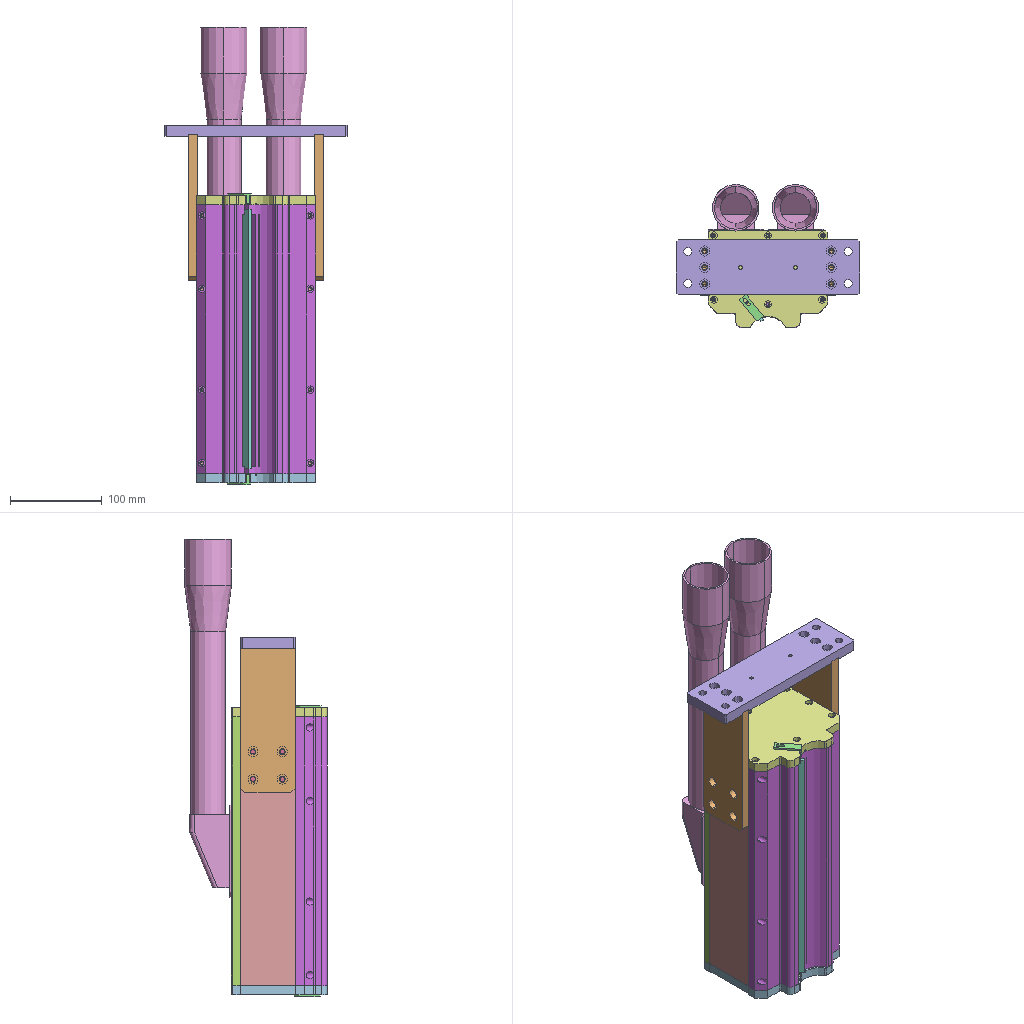Assembly | SolidWorks | 12 different items | 16 placed | box 200 x 156 x 499 mm
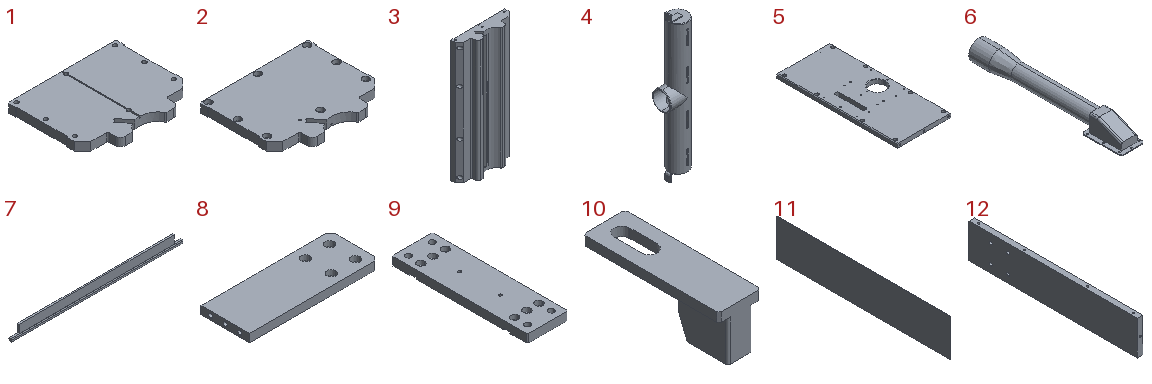Parts list (item | quantity | size | volume | features):
1 | x1 | 130 x 105 x 10 mm | 118021 mm3 | features ICE 5, Fillet 3, Chamfer 2, HoleWzd 2, Extrusion 1
2 | x1 | 130 x 105 x 10 mm | 118021 mm3 | features ICE 5, Fillet 3, Chamfer 2, HoleWzd 2, Extrusion 1
3 | x1 | 130 x 35 x 293 mm | 778685 mm3 | features ICE 4, Fillet 3, HoleWzd 2, MirrorPattern 2, Chamfer 1, Cut 1, Extrusion 1, LPattern 1
4 | x1 | 52 x 38 x 290 mm | 64495 mm3 | features Fillet 4, ICE 4, Chamfer 3, MirrorPattern 2, Extrusion 1, Shell 1
5 | x1 | 130 x 293 x 10 mm | 356054 mm3 | features HoleWzd 5, MirrorPattern 4, Chamfer 2, Cut 2, Extrusion 1, ICE 1
6 | x2 | 60 x 390 x 51 mm | 98660 mm3 | features ICE 4, Chamfer 1, Cut 1, Extrusion 1, Fillet 1, MirrorPattern 1, Revolution 1, Shell 1
7 | x1 | 313 x 5 x 20.5 mm | 20756 mm3 | features ICE 2, Extrusion 1
8 | x2 | 160 x 60 x 10 mm | 92147 mm3 | features HoleWzd 2, Chamfer 1, Extrusion 1
9 | x1 | 60 x 200 x 12 mm | 134076 mm3 | features Cut 2, Chamfer 1, Extrusion 1, HoleWzd 1, ICE 1
10 | x2 | 9.3 x 30 x 11 mm | 992.992 mm3 | features Chamfer 2, ICE 2, Extrusion 1, Fillet 1
11 | x1 | 1.5 x 297 x 64 mm | 28512 mm3 | features Extrusion 1
12 | x2 | 10 x 293 x 60 mm | 174003 mm3 | features HoleWzd 3, MirrorPattern 2, Extrusion 1
Mates (type | each side: item.copy, entity, surface, feature):
Coincident | 3.1 plane | 11.1 plane
Coincident | 3.1 face plane Boss-Extrude1 | 12.1 face plane Boss-Extrude1
Coincident | 3.1 face plane Boss-Extrude1 | 12.2 face plane Boss-Extrude1
Coincident | 3.1 face plane Boss-Extrude1 | 2.1 face plane Boss-Extrude1
Coincident | 3.1 plane | 4.1 plane
Coincident | 3.1 face plane Boss-Extrude1 | 1.1 face plane Boss-Extrude1
Coincident | 12.1 face plane Boss-Extrude1 | 5.1 face plane Boss-Extrude1 | 2 times
Coincident | 5.1 face plane Boss-Extrude1 | 6.1 face plane Boss-Extrude1
Coincident | 1.1 face plane Cut-Extrude8 | 7.1 face plane Boss-Extrude1 | 2 times
Coincident | 1.1 face plane Boss-Extrude1 | 7.1 face plane Boss-Extrude1
Coincident | 1.1 plane | 9.1 plane
Coincident | 2.1 face plane Boss-Extrude1 | 5.1 face plane Boss-Extrude1
Coincident | 2.1 face plane Cut-Extrude8 | 10.1 face plane Boss-Extrude1
Coincident | 2.1 face plane Boss-Extrude1 | 10.1 face plane Boss-Extrude2
Coincident | 5.1 plane | 6.1 plane
Coincident | 5.1 face plane Boss-Extrude1 | 6.1 face plane Boss-Extrude3
Coincident | 1.1 face plane Boss-Extrude1 | 10.2 face plane Boss-Extrude2
Coincident | 1.1 face plane Cut-Extrude8 | 10.2 face plane Boss-Extrude1
Coincident | 7.1 face plane Boss-Extrude1 | 10.2 face plane Boss-Extrude1
Coincident | 12.1 face plane Boss-Extrude1 | 2.1 face plane Boss-Extrude1
DistanceDim | 12.1 face plane Boss-Extrude1 | 3.1 face plane Boss-Extrude1
Coincident | 12.2 face plane Boss-Extrude1 | 2.1 face plane Boss-Extrude1
DistanceDim | 12.2 face plane Boss-Extrude1 | 3.1 face plane Boss-Extrude1
Coincident | 5.1 face plane Cut-Extrude3 | 11.1 face plane Boss-Extrude1
DistanceDim | 11.1 face plane Boss-Extrude1 | 5.1 face plane Boss-Extrude1
Coincident | 12.1 face plane Boss-Extrude1 | 8.1 face plane Boss-Extrude1
Concentric | 12.1 face cylinder M6 Tapped Hole1 | 8.1 face cylinder CBORE for M6 Hex Socket Head Cap Screw1 | 2 times
Coincident | 12.2 face plane Boss-Extrude1 | 8.2 face plane Boss-Extrude1
Concentric | 12.2 face cylinder M6 Tapped Hole1 | 8.2 face cylinder CBORE for M6 Hex Socket Head Cap Screw1 | 2 times
Coincident | 8.2 face plane Boss-Extrude1 | 9.1 face plane Cut-Extrude1
Coincident | 8.2 face plane Boss-Extrude1 | 9.1 face plane Boss-Extrude1